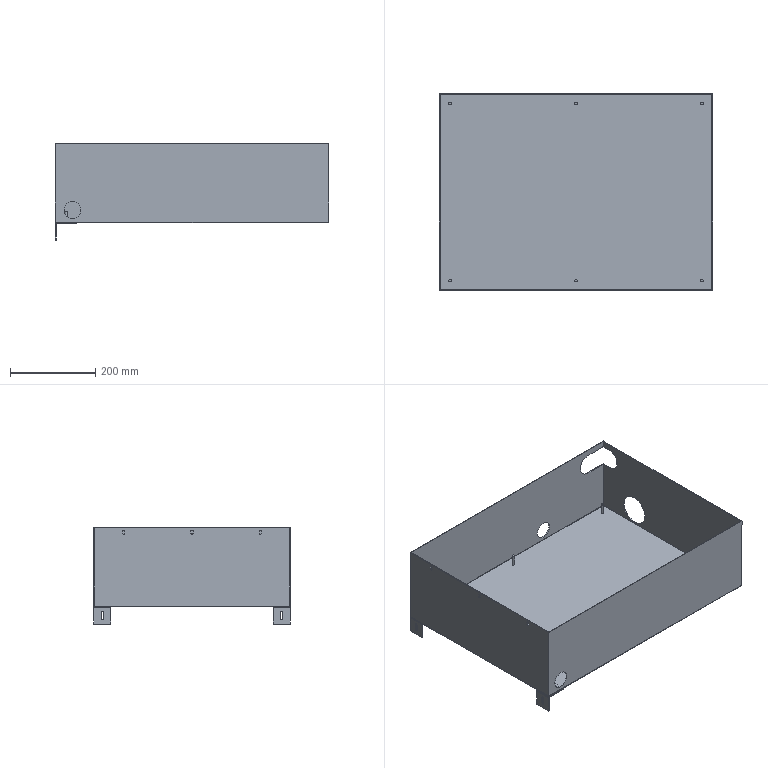Part | STEP file | CS-DS-001 | 3 solids | 131 faces | box 640 x 460 x 225 mm | volume 1382165 mm3 | plane 76 | cylinder 47 | spline 8 | commonest cylinder face diameters 6 x12 5.8 x9 0.4 x6 4.4 x6 5.5 x6 40 x4